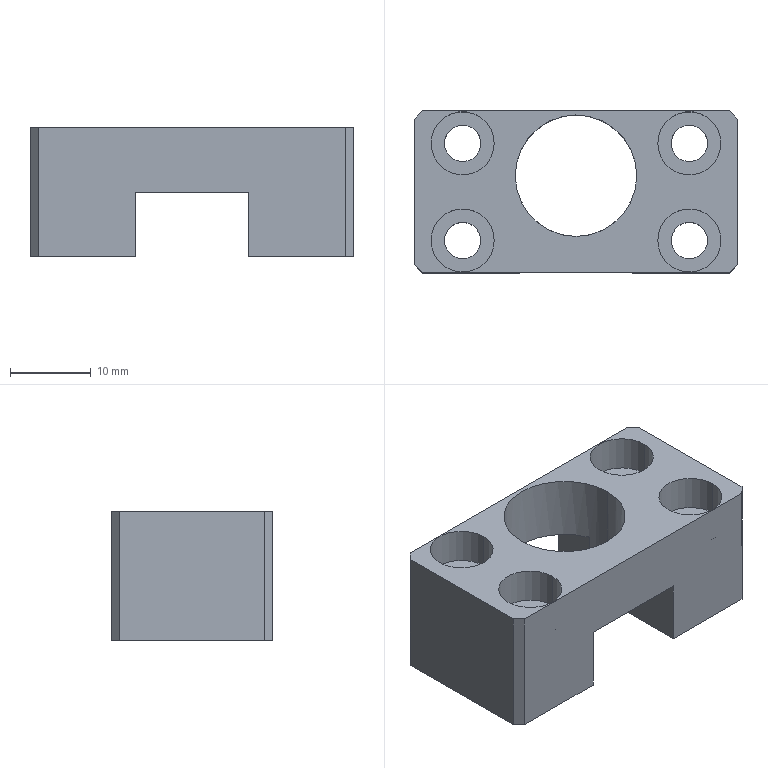Part | SolidWorks | features HoleWzd 2, Chamfer 1, Extrusion 1, ICE 1 | 1 solid | 39 faces | box 40 x 20 x 16 mm | volume 7506 mm3 | plane 21 | cylinder 18 | commonest cylinder face diameters 4.5 x8 7.8 x8 15 x2
STEP:
#1=CARTESIAN_POINT('',(10.1,6.,3.6));
#2=VERTEX_POINT('',#1);
#3=CARTESIAN_POINT('',(17.9,6.,3.6));
#4=VERTEX_POINT('',#3);
#5=CARTESIAN_POINT('',(14.,6.,3.6));
#6=DIRECTION('',(0.,0.,1.));
#7=DIRECTION('',(1.,0.,0.));
#8=AXIS2_PLACEMENT_3D('',#5,#6,#7);
#9=CIRCLE('',#8,3.9);
#10=EDGE_CURVE('',#2,#4,#9,.T.);
#11=ORIENTED_EDGE('',*,*,#10,.F.);
#12=CARTESIAN_POINT('',(10.1,6.,8.));
#13=VERTEX_POINT('',#12);
#14=CARTESIAN_POINT('',(10.1,6.,8.));
#15=DIRECTION('',(0.,0.,1.));
#16=VECTOR('',#15,1000.);
#17=LINE('',#14,#16);
#18=EDGE_CURVE('',#2,#13,#17,.T.);
#19=ORIENTED_EDGE('',*,*,#18,.T.);
#20=CARTESIAN_POINT('',(17.9,6.,8.));
#21=VERTEX_POINT('',#20);
#22=CARTESIAN_POINT('',(14.,6.,8.));
#23=DIRECTION('',(0.,0.,1.));
#24=DIRECTION('',(1.,0.,0.));
#25=AXIS2_PLACEMENT_3D('',#22,#23,#24);
#26=CIRCLE('',#25,3.9);
#27=EDGE_CURVE('',#13,#21,#26,.T.);
#28=ORIENTED_EDGE('',*,*,#27,.T.);
#29=CARTESIAN_POINT('',(17.9,6.,8.));
#30=DIRECTION('',(0.,0.,1.));
#31=VECTOR('',#30,1000.);
#32=LINE('',#29,#31);
#33=EDGE_CURVE('',#4,#21,#32,.T.);
#34=ORIENTED_EDGE('',*,*,#33,.F.);
#35=EDGE_LOOP('',(#11,#19,#28,#34));
#36=FACE_OUTER_BOUND('',#35,.T.);
#37=CARTESIAN_POINT('',(14.,6.,8.));
#38=DIRECTION('',(0.,0.,1.));
#39=DIRECTION('',(1.,0.,0.));
#40=AXIS2_PLACEMENT_3D('',#37,#38,#39);
#41=CYLINDRICAL_SURFACE('',#40,3.9);
#42=ADVANCED_FACE('',(#36),#41,.F.);
#43=CARTESIAN_POINT('',(11.75,6.,-8.));
#44=VERTEX_POINT('',#43);
#45=CARTESIAN_POINT('',(16.25,6.,-8.));
#46=VERTEX_POINT('',#45);
#47=CARTESIAN_POINT('',(14.,6.,-8.));
#48=DIRECTION('',(0.,0.,1.));
#49=DIRECTION('',(1.,0.,0.));
#50=AXIS2_PLACEMENT_3D('',#47,#48,#49);
#51=CIRCLE('',#50,2.25);
#52=EDGE_CURVE('',#44,#46,#51,.T.);
#53=ORIENTED_EDGE('',*,*,#52,.F.);
#54=CARTESIAN_POINT('',(11.75,6.,3.6));
#55=VERTEX_POINT('',#54);
#56=CARTESIAN_POINT('',(11.75,6.,8.));
#57=DIRECTION('',(0.,0.,1.));
#58=VECTOR('',#57,1000.);
#59=LINE('',#56,#58);
#60=EDGE_CURVE('',#44,#55,#59,.T.);
#61=ORIENTED_EDGE('',*,*,#60,.T.);
#62=CARTESIAN_POINT('',(16.25,6.,3.6));
#63=VERTEX_POINT('',#62);
#64=CARTESIAN_POINT('',(14.,6.,3.6));
#65=DIRECTION('',(0.,0.,1.));
#66=DIRECTION('',(1.,0.,0.));
#67=AXIS2_PLACEMENT_3D('',#64,#65,#66);
#68=CIRCLE('',#67,2.25);
#69=EDGE_CURVE('',#55,#63,#68,.T.);
#70=ORIENTED_EDGE('',*,*,#69,.T.);
#71=CARTESIAN_POINT('',(16.25,6.,8.));
#72=DIRECTION('',(0.,0.,1.));
#73=VECTOR('',#72,1000.);
#74=LINE('',#71,#73);
#75=EDGE_CURVE('',#46,#63,#74,.T.);
#76=ORIENTED_EDGE('',*,*,#75,.F.);
#77=EDGE_LOOP('',(#53,#61,#70,#76));
#78=FACE_OUTER_BOUND('',#77,.T.);
#79=CARTESIAN_POINT('',(14.,6.,8.));
#80=DIRECTION('',(0.,0.,1.));
#81=DIRECTION('',(1.,0.,0.));
#82=AXIS2_PLACEMENT_3D('',#79,#80,#81);
#83=CYLINDRICAL_SURFACE('',#82,2.25);
#84=ADVANCED_FACE('',(#78),#83,.F.);
#85=CARTESIAN_POINT('',(-17.9,-6.,3.6));
#86=VERTEX_POINT('',#85);
#87=CARTESIAN_POINT('',(-10.1,-6.,3.6));
#88=VERTEX_POINT('',#87);
#89=CARTESIAN_POINT('',(-14.,-6.,3.6));
#90=DIRECTION('',(0.,0.,1.));
#91=DIRECTION('',(1.,0.,0.));
#92=AXIS2_PLACEMENT_3D('',#89,#90,#91);
#93=CIRCLE('',#92,3.9);
#94=EDGE_CURVE('',#86,#88,#93,.T.);
#95=ORIENTED_EDGE('',*,*,#94,.F.);
#96=CARTESIAN_POINT('',(-17.9,-6.,8.));
#97=VERTEX_POINT('',#96);
#98=CARTESIAN_POINT('',(-17.9,-6.,8.));
#99=DIRECTION('',(0.,0.,1.));
#100=VECTOR('',#99,1000.);
#101=LINE('',#98,#100);
#102=EDGE_CURVE('',#86,#97,#101,.T.);
#103=ORIENTED_EDGE('',*,*,#102,.T.);
#104=CARTESIAN_POINT('',(-10.1,-6.,8.));
#105=VERTEX_POINT('',#104);
#106=CARTESIAN_POINT('',(-14.,-6.,8.));
#107=DIRECTION('',(0.,0.,1.));
#108=DIRECTION('',(1.,0.,0.));
#109=AXIS2_PLACEMENT_3D('',#106,#107,#108);
#110=CIRCLE('',#109,3.9);
#111=EDGE_CURVE('',#97,#105,#110,.T.);
#112=ORIENTED_EDGE('',*,*,#111,.T.);
#113=CARTESIAN_POINT('',(-10.1,-6.,8.));
#114=DIRECTION('',(0.,0.,1.));
#115=VECTOR('',#114,1000.);
#116=LINE('',#113,#115);
#117=EDGE_CURVE('',#88,#105,#116,.T.);
#118=ORIENTED_EDGE('',*,*,#117,.F.);
#119=EDGE_LOOP('',(#95,#103,#112,#118));
#120=FACE_OUTER_BOUND('',#119,.T.);
#121=CARTESIAN_POINT('',(-14.,-6.,8.));
#122=DIRECTION('',(0.,0.,1.));
#123=DIRECTION('',(1.,0.,0.));
#124=AXIS2_PLACEMENT_3D('',#121,#122,#123);
#125=CYLINDRICAL_SURFACE('',#124,3.9);
#126=ADVANCED_FACE('',(#120),#125,.F.);
#127=CARTESIAN_POINT('',(-16.25,-6.,-8.));
#128=VERTEX_POINT('',#127);
#129=CARTESIAN_POINT('',(-11.75,-6.,-8.));
#130=VERTEX_POINT('',#129);
#131=CARTESIAN_POINT('',(-14.,-6.,-8.));
#132=DIRECTION('',(0.,0.,1.));
#133=DIRECTION('',(1.,0.,0.));
#134=AXIS2_PLACEMENT_3D('',#131,#132,#133);
#135=CIRCLE('',#134,2.25);
#136=EDGE_CURVE('',#128,#130,#135,.T.);
#137=ORIENTED_EDGE('',*,*,#136,.F.);
#138=CARTESIAN_POINT('',(-16.25,-6.,3.6));
#139=VERTEX_POINT('',#138);
#140=CARTESIAN_POINT('',(-16.25,-6.,8.));
#141=DIRECTION('',(0.,0.,1.));
#142=VECTOR('',#141,1000.);
#143=LINE('',#140,#142);
#144=EDGE_CURVE('',#128,#139,#143,.T.);
#145=ORIENTED_EDGE('',*,*,#144,.T.);
#146=CARTESIAN_POINT('',(-11.75,-6.,3.6));
#147=VERTEX_POINT('',#146);
#148=CARTESIAN_POINT('',(-14.,-6.,3.6));
#149=DIRECTION('',(0.,0.,1.));
#150=DIRECTION('',(1.,0.,0.));
#151=AXIS2_PLACEMENT_3D('',#148,#149,#150);
#152=CIRCLE('',#151,2.25);
#153=EDGE_CURVE('',#139,#147,#152,.T.);
#154=ORIENTED_EDGE('',*,*,#153,.T.);
#155=CARTESIAN_POINT('',(-11.75,-6.,8.));
#156=DIRECTION('',(0.,0.,1.));
#157=VECTOR('',#156,1000.);
#158=LINE('',#155,#157);
#159=EDGE_CURVE('',#130,#147,#158,.T.);
#160=ORIENTED_EDGE('',*,*,#159,.F.);
#161=EDGE_LOOP('',(#137,#145,#154,#160));
#162=FACE_OUTER_BOUND('',#161,.T.);
#163=CARTESIAN_POINT('',(-14.,-6.,8.));
#164=DIRECTION('',(0.,0.,1.));
#165=DIRECTION('',(1.,0.,0.));
#166=AXIS2_PLACEMENT_3D('',#163,#164,#165);
#167=CYLINDRICAL_SURFACE('',#166,2.25);
#168=ADVANCED_FACE('',(#162),#167,.F.);
#169=CARTESIAN_POINT('',(-17.9,6.,3.6));
#170=VERTEX_POINT('',#169);
#171=CARTESIAN_POINT('',(-10.1,6.,3.6));
#172=VERTEX_POINT('',#171);
#173=CARTESIAN_POINT('',(-14.,6.,3.6));
#174=DIRECTION('',(0.,0.,1.));
#175=DIRECTION('',(1.,0.,0.));
#176=AXIS2_PLACEMENT_3D('',#173,#174,#175);
#177=CIRCLE('',#176,3.9);
#178=EDGE_CURVE('',#170,#172,#177,.T.);
#179=ORIENTED_EDGE('',*,*,#178,.F.);
#180=CARTESIAN_POINT('',(-17.9,6.,8.));
#181=VERTEX_POINT('',#180);
#182=CARTESIAN_POINT('',(-17.9,6.,8.));
#183=DIRECTION('',(0.,0.,1.));
#184=VECTOR('',#183,1000.);
#185=LINE('',#182,#184);
#186=EDGE_CURVE('',#170,#181,#185,.T.);
#187=ORIENTED_EDGE('',*,*,#186,.T.);
#188=CARTESIAN_POINT('',(-10.1,6.,8.));
#189=VERTEX_POINT('',#188);
#190=CARTESIAN_POINT('',(-14.,6.,8.));
#191=DIRECTION('',(0.,0.,1.));
#192=DIRECTION('',(1.,0.,0.));
#193=AXIS2_PLACEMENT_3D('',#190,#191,#192);
#194=CIRCLE('',#193,3.9);
#195=EDGE_CURVE('',#181,#189,#194,.T.);
#196=ORIENTED_EDGE('',*,*,#195,.T.);
#197=CARTESIAN_POINT('',(-10.1,6.,8.));
#198=DIRECTION('',(0.,0.,1.));
#199=VECTOR('',#198,1000.);
#200=LINE('',#197,#199);
#201=EDGE_CURVE('',#172,#189,#200,.T.);
#202=ORIENTED_EDGE('',*,*,#201,.F.);
#203=EDGE_LOOP('',(#179,#187,#196,#202));
#204=FACE_OUTER_BOUND('',#203,.T.);
#205=CARTESIAN_POINT('',(-14.,6.,8.));
#206=DIRECTION('',(0.,0.,1.));
#207=DIRECTION('',(1.,0.,0.));
#208=AXIS2_PLACEMENT_3D('',#205,#206,#207);
#209=CYLINDRICAL_SURFACE('',#208,3.9);
#210=ADVANCED_FACE('',(#204),#209,.F.);
#211=CARTESIAN_POINT('',(-16.25,6.,-8.));
#212=VERTEX_POINT('',#211);
#213=CARTESIAN_POINT('',(-11.75,6.,-8.));
#214=VERTEX_POINT('',#213);
#215=CARTESIAN_POINT('',(-14.,6.,-8.));
#216=DIRECTION('',(0.,0.,1.));
#217=DIRECTION('',(1.,0.,0.));
#218=AXIS2_PLACEMENT_3D('',#215,#216,#217);
#219=CIRCLE('',#218,2.25);
#220=EDGE_CURVE('',#212,#214,#219,.T.);
#221=ORIENTED_EDGE('',*,*,#220,.F.);
#222=CARTESIAN_POINT('',(-16.25,6.,3.6));
#223=VERTEX_POINT('',#222);
#224=CARTESIAN_POINT('',(-16.25,6.,8.));
#225=DIRECTION('',(0.,0.,1.));
#226=VECTOR('',#225,1000.);
#227=LINE('',#224,#226);
#228=EDGE_CURVE('',#212,#223,#227,.T.);
#229=ORIENTED_EDGE('',*,*,#228,.T.);
#230=CARTESIAN_POINT('',(-11.75,6.,3.6));
#231=VERTEX_POINT('',#230);
#232=CARTESIAN_POINT('',(-14.,6.,3.6));
#233=DIRECTION('',(0.,0.,1.));
#234=DIRECTION('',(1.,0.,0.));
#235=AXIS2_PLACEMENT_3D('',#232,#233,#234);
#236=CIRCLE('',#235,2.25);
#237=EDGE_CURVE('',#223,#231,#236,.T.);
#238=ORIENTED_EDGE('',*,*,#237,.T.);
#239=CARTESIAN_POINT('',(-11.75,6.,8.));
#240=DIRECTION('',(0.,0.,1.));
#241=VECTOR('',#240,1000.);
#242=LINE('',#239,#241);
#243=EDGE_CURVE('',#214,#231,#242,.T.);
#244=ORIENTED_EDGE('',*,*,#243,.F.);
#245=EDGE_LOOP('',(#221,#229,#238,#244));
#246=FACE_OUTER_BOUND('',#245,.T.);
#247=CARTESIAN_POINT('',(-14.,6.,8.));
#248=DIRECTION('',(0.,0.,1.));
#249=DIRECTION('',(1.,0.,0.));
#250=AXIS2_PLACEMENT_3D('',#247,#248,#249);
#251=CYLINDRICAL_SURFACE('',#250,2.25);
#252=ADVANCED_FACE('',(#246),#251,.F.);
#253=CARTESIAN_POINT('',(10.1,-6.,3.6));
#254=VERTEX_POINT('',#253);
#255=CARTESIAN_POINT('',(17.9,-6.,3.6));
#256=VERTEX_POINT('',#255);
#257=CARTESIAN_POINT('',(14.,-6.,3.6));
#258=DIRECTION('',(0.,0.,1.));
#259=DIRECTION('',(1.,0.,0.));
#260=AXIS2_PLACEMENT_3D('',#257,#258,#259);
#261=CIRCLE('',#260,3.9);
#262=EDGE_CURVE('',#254,#256,#261,.T.);
#263=ORIENTED_EDGE('',*,*,#262,.F.);
#264=CARTESIAN_POINT('',(10.1,-6.,8.));
#265=VERTEX_POINT('',#264);
#266=CARTESIAN_POINT('',(10.1,-6.,8.));
#267=DIRECTION('',(0.,0.,1.));
#268=VECTOR('',#267,1000.);
#269=LINE('',#266,#268);
#270=EDGE_CURVE('',#254,#265,#269,.T.);
#271=ORIENTED_EDGE('',*,*,#270,.T.);
#272=CARTESIAN_POINT('',(17.9,-6.,8.));
#273=VERTEX_POINT('',#272);
#274=CARTESIAN_POINT('',(14.,-6.,8.));
#275=DIRECTION('',(0.,0.,1.));
#276=DIRECTION('',(1.,0.,0.));
#277=AXIS2_PLACEMENT_3D('',#274,#275,#276);
#278=CIRCLE('',#277,3.9);
#279=EDGE_CURVE('',#265,#273,#278,.T.);
#280=ORIENTED_EDGE('',*,*,#279,.T.);
#281=CARTESIAN_POINT('',(17.9,-6.,8.));
#282=DIRECTION('',(0.,0.,1.));
#283=VECTOR('',#282,1000.);
#284=LINE('',#281,#283);
#285=EDGE_CURVE('',#256,#273,#284,.T.);
#286=ORIENTED_EDGE('',*,*,#285,.F.);
#287=EDGE_LOOP('',(#263,#271,#280,#286));
#288=FACE_OUTER_BOUND('',#287,.T.);
#289=CARTESIAN_POINT('',(14.,-6.,8.));
#290=DIRECTION('',(0.,0.,1.));
#291=DIRECTION('',(1.,0.,0.));
#292=AXIS2_PLACEMENT_3D('',#289,#290,#291);
#293=CYLINDRICAL_SURFACE('',#292,3.9);
#294=ADVANCED_FACE('',(#288),#293,.F.);
#295=CARTESIAN_POINT('',(11.75,-6.,-8.));
#296=VERTEX_POINT('',#295);
#297=CARTESIAN_POINT('',(16.25,-6.,-8.));
#298=VERTEX_POINT('',#297);
#299=CARTESIAN_POINT('',(14.,-6.,-8.));
#300=DIRECTION('',(0.,0.,1.));
#301=DIRECTION('',(1.,0.,0.));
#302=AXIS2_PLACEMENT_3D('',#299,#300,#301);
#303=CIRCLE('',#302,2.25);
#304=EDGE_CURVE('',#296,#298,#303,.T.);
#305=ORIENTED_EDGE('',*,*,#304,.F.);
#306=CARTESIAN_POINT('',(11.75,-6.,3.6));
#307=VERTEX_POINT('',#306);
#308=CARTESIAN_POINT('',(11.75,-6.,8.));
#309=DIRECTION('',(0.,0.,1.));
#310=VECTOR('',#309,1000.);
#311=LINE('',#308,#310);
#312=EDGE_CURVE('',#296,#307,#311,.T.);
#313=ORIENTED_EDGE('',*,*,#312,.T.);
#314=CARTESIAN_POINT('',(16.25,-6.,3.6));
#315=VERTEX_POINT('',#314);
#316=CARTESIAN_POINT('',(14.,-6.,3.6));
#317=DIRECTION('',(0.,0.,1.));
#318=DIRECTION('',(1.,0.,0.));
#319=AXIS2_PLACEMENT_3D('',#316,#317,#318);
#320=CIRCLE('',#319,2.25);
#321=EDGE_CURVE('',#307,#315,#320,.T.);
#322=ORIENTED_EDGE('',*,*,#321,.T.);
#323=CARTESIAN_POINT('',(16.25,-6.,8.));
#324=DIRECTION('',(0.,0.,1.));
#325=VECTOR('',#324,1000.);
#326=LINE('',#323,#325);
#327=EDGE_CURVE('',#298,#315,#326,.T.);
#328=ORIENTED_EDGE('',*,*,#327,.F.);
#329=EDGE_LOOP('',(#305,#313,#322,#328));
#330=FACE_OUTER_BOUND('',#329,.T.);
#331=CARTESIAN_POINT('',(14.,-6.,8.));
#332=DIRECTION('',(0.,0.,1.));
#333=DIRECTION('',(1.,0.,0.));
#334=AXIS2_PLACEMENT_3D('',#331,#332,#333);
#335=CYLINDRICAL_SURFACE('',#334,2.25);
#336=ADVANCED_FACE('',(#330),#335,.F.);
#337=CARTESIAN_POINT('',(-7.,-0.6926,-8.));
#338=VERTEX_POINT('',#337);
#339=CARTESIAN_POINT('',(-7.5,2.,-8.));
#340=VERTEX_POINT('',#339);
#341=CARTESIAN_POINT('',(0.,2.,-8.));
#342=DIRECTION('',(0.,0.,-1.));
#343=DIRECTION('',(-1.,0.,0.));
#344=AXIS2_PLACEMENT_3D('',#341,#342,#343);
#345=CIRCLE('',#344,7.5);
#346=EDGE_CURVE('',#338,#340,#345,.T.);
#347=ORIENTED_EDGE('',*,*,#346,.T.);
#348=CARTESIAN_POINT('',(-7.5,2.,8.));
#349=VERTEX_POINT('',#348);
#350=CARTESIAN_POINT('',(-7.5,2.,8.));
#351=DIRECTION('',(0.,0.,1.));
#352=VECTOR('',#351,1000.);
#353=LINE('',#350,#352);
#354=EDGE_CURVE('',#340,#349,#353,.T.);
#355=ORIENTED_EDGE('',*,*,#354,.T.);
#356=CARTESIAN_POINT('',(7.5,2.,8.));
#357=VERTEX_POINT('',#356);
#358=CARTESIAN_POINT('',(0.,2.,8.));
#359=DIRECTION('',(0.,0.,1.));
#360=DIRECTION('',(1.,0.,0.));
#361=AXIS2_PLACEMENT_3D('',#358,#359,#360);
#362=CIRCLE('',#361,7.5);
#363=EDGE_CURVE('',#349,#357,#362,.T.);
#364=ORIENTED_EDGE('',*,*,#363,.T.);
#365=CARTESIAN_POINT('',(7.5,2.,-8.));
#366=VERTEX_POINT('',#365);
#367=CARTESIAN_POINT('',(7.5,2.,8.));
#368=DIRECTION('',(0.,0.,1.));
#369=VECTOR('',#368,1000.);
#370=LINE('',#367,#369);
#371=EDGE_CURVE('',#366,#357,#370,.T.);
#372=ORIENTED_EDGE('',*,*,#371,.F.);
#373=CARTESIAN_POINT('',(7.,-0.6926,-8.));
#374=VERTEX_POINT('',#373);
#375=CARTESIAN_POINT('',(0.,2.,-8.));
#376=DIRECTION('',(0.,0.,-1.));
#377=DIRECTION('',(-1.,0.,0.));
#378=AXIS2_PLACEMENT_3D('',#375,#376,#377);
#379=CIRCLE('',#378,7.5);
#380=EDGE_CURVE('',#366,#374,#379,.T.);
#381=ORIENTED_EDGE('',*,*,#380,.T.);
#382=CARTESIAN_POINT('',(7.,-0.6926,0.));
#383=VERTEX_POINT('',#382);
#384=CARTESIAN_POINT('',(7.,-0.6926,8.));
#385=DIRECTION('',(0.,0.,1.));
#386=VECTOR('',#385,1000.);
#387=LINE('',#384,#386);
#388=EDGE_CURVE('',#374,#383,#387,.T.);
#389=ORIENTED_EDGE('',*,*,#388,.T.);
#390=CARTESIAN_POINT('',(-7.,-0.6926,0.));
#391=VERTEX_POINT('',#390);
#392=CARTESIAN_POINT('',(0.,2.,0.));
#393=DIRECTION('',(0.,0.,1.));
#394=DIRECTION('',(-1.,0.,0.));
#395=AXIS2_PLACEMENT_3D('',#392,#393,#394);
#396=CIRCLE('',#395,7.5);
#397=EDGE_CURVE('',#391,#383,#396,.T.);
#398=ORIENTED_EDGE('',*,*,#397,.F.);
#399=CARTESIAN_POINT('',(-7.,-0.6926,8.));
#400=DIRECTION('',(0.,0.,-1.));
#401=VECTOR('',#400,1000.);
#402=LINE('',#399,#401);
#403=EDGE_CURVE('',#391,#338,#402,.T.);
#404=ORIENTED_EDGE('',*,*,#403,.T.);
#405=EDGE_LOOP('',(#347,#355,#364,#372,#381,#389,#398,#404));
#406=FACE_OUTER_BOUND('',#405,.T.);
#407=CARTESIAN_POINT('',(0.,2.,8.));
#408=DIRECTION('',(0.,0.,1.));
#409=DIRECTION('',(1.,0.,0.));
#410=AXIS2_PLACEMENT_3D('',#407,#408,#409);
#411=CYLINDRICAL_SURFACE('',#410,7.5);
#412=ADVANCED_FACE('',(#406),#411,.F.);
#413=CARTESIAN_POINT('',(-14.,-6.,-8.));
#414=DIRECTION('',(0.,0.,1.));
#415=DIRECTION('',(1.,0.,0.));
#416=AXIS2_PLACEMENT_3D('',#413,#414,#415);
#417=CIRCLE('',#416,2.25);
#418=EDGE_CURVE('',#130,#128,#417,.T.);
#419=ORIENTED_EDGE('',*,*,#418,.T.);
#420=ORIENTED_EDGE('',*,*,#136,.T.);
#421=EDGE_LOOP('',(#419,#420));
#422=FACE_BOUND('',#421,.T.);
#423=CARTESIAN_POINT('',(-14.,6.,-8.));
#424=DIRECTION('',(0.,0.,1.));
#425=DIRECTION('',(1.,0.,0.));
#426=AXIS2_PLACEMENT_3D('',#423,#424,#425);
#427=CIRCLE('',#426,2.25);
#428=EDGE_CURVE('',#214,#212,#427,.T.);
#429=ORIENTED_EDGE('',*,*,#428,.T.);
#430=ORIENTED_EDGE('',*,*,#220,.T.);
#431=EDGE_LOOP('',(#429,#430));
#432=FACE_BOUND('',#431,.T.);
#433=CARTESIAN_POINT('',(-7.,-10.,-8.));
#434=VERTEX_POINT('',#433);
#435=CARTESIAN_POINT('',(-7.,-15.772,-8.));
#436=DIRECTION('',(0.,1.,0.));
#437=VECTOR('',#436,1000.);
#438=LINE('',#435,#437);
#439=EDGE_CURVE('',#434,#338,#438,.T.);
#440=ORIENTED_EDGE('',*,*,#439,.F.);
#441=CARTESIAN_POINT('',(-19.,-10.,-8.));
#442=VERTEX_POINT('',#441);
#443=CARTESIAN_POINT('',(-20.,-10.,-8.));
#444=DIRECTION('',(1.,0.,0.));
#445=VECTOR('',#444,1000.);
#446=LINE('',#443,#445);
#447=EDGE_CURVE('',#442,#434,#446,.T.);
#448=ORIENTED_EDGE('',*,*,#447,.F.);
#449=CARTESIAN_POINT('',(-20.,-9.,-8.));
#450=VERTEX_POINT('',#449);
#451=CARTESIAN_POINT('',(-14.5,-14.5,-8.));
#452=DIRECTION('',(-0.7071,0.7071,0.));
#453=VECTOR('',#452,1000.);
#454=LINE('',#451,#453);
#455=EDGE_CURVE('',#442,#450,#454,.T.);
#456=ORIENTED_EDGE('',*,*,#455,.T.);
#457=CARTESIAN_POINT('',(-20.,9.,-8.));
#458=VERTEX_POINT('',#457);
#459=CARTESIAN_POINT('',(-20.,-10.,-8.));
#460=DIRECTION('',(0.,-1.,0.));
#461=VECTOR('',#460,1000.);
#462=LINE('',#459,#461);
#463=EDGE_CURVE('',#458,#450,#462,.T.);
#464=ORIENTED_EDGE('',*,*,#463,.F.);
#465=CARTESIAN_POINT('',(-19.,10.,-8.));
#466=VERTEX_POINT('',#465);
#467=CARTESIAN_POINT('',(-14.5,14.5,-8.));
#468=DIRECTION('',(0.7071,0.7071,0.));
#469=VECTOR('',#468,1000.);
#470=LINE('',#467,#469);
#471=EDGE_CURVE('',#458,#466,#470,.T.);
#472=ORIENTED_EDGE('',*,*,#471,.T.);
#473=CARTESIAN_POINT('',(-7.,10.,-8.));
#474=VERTEX_POINT('',#473);
#475=CARTESIAN_POINT('',(-20.,10.,-8.));
#476=DIRECTION('',(-1.,0.,0.));
#477=VECTOR('',#476,1000.);
#478=LINE('',#475,#477);
#479=EDGE_CURVE('',#474,#466,#478,.T.);
#480=ORIENTED_EDGE('',*,*,#479,.F.);
#481=CARTESIAN_POINT('',(-7.,4.693,-8.));
#482=VERTEX_POINT('',#481);
#483=CARTESIAN_POINT('',(-7.,-15.772,-8.));
#484=DIRECTION('',(0.,1.,0.));
#485=VECTOR('',#484,1000.);
#486=LINE('',#483,#485);
#487=EDGE_CURVE('',#482,#474,#486,.T.);
#488=ORIENTED_EDGE('',*,*,#487,.F.);
#489=CARTESIAN_POINT('',(0.,2.,-8.));
#490=DIRECTION('',(0.,0.,-1.));
#491=DIRECTION('',(-1.,0.,0.));
#492=AXIS2_PLACEMENT_3D('',#489,#490,#491);
#493=CIRCLE('',#492,7.5);
#494=EDGE_CURVE('',#340,#482,#493,.T.);
#495=ORIENTED_EDGE('',*,*,#494,.F.);
#496=ORIENTED_EDGE('',*,*,#346,.F.);
#497=EDGE_LOOP('',(#440,#448,#456,#464,#472,#480,#488,#495,#496));
#498=FACE_OUTER_BOUND('',#497,.T.);
#499=CARTESIAN_POINT('',(0.,0.,-8.));
#500=DIRECTION('',(0.,0.,-1.));
#501=DIRECTION('',(-1.,0.,0.));
#502=AXIS2_PLACEMENT_3D('',#499,#500,#501);
#503=PLANE('',#502);
#504=ADVANCED_FACE('',(#422,#432,#498),#503,.T.);
#505=CARTESIAN_POINT('',(20.,-9.,8.));
#506=VERTEX_POINT('',#505);
#507=CARTESIAN_POINT('',(20.,9.,8.));
#508=VERTEX_POINT('',#507);
#509=CARTESIAN_POINT('',(20.,-10.,8.));
#510=DIRECTION('',(0.,1.,0.));
#511=VECTOR('',#510,1000.);
#512=LINE('',#509,#511);
#513=EDGE_CURVE('',#506,#508,#512,.T.);
#514=ORIENTED_EDGE('',*,*,#513,.F.);
#515=CARTESIAN_POINT('',(20.,-9.,-8.));
#516=VERTEX_POINT('',#515);
#517=CARTESIAN_POINT('',(20.,-9.,8.));
#518=DIRECTION('',(0.,0.,-1.));
#519=VECTOR('',#518,1000.);
#520=LINE('',#517,#519);
#521=EDGE_CURVE('',#506,#516,#520,.T.);
#522=ORIENTED_EDGE('',*,*,#521,.T.);
#523=CARTESIAN_POINT('',(20.,9.,-8.));
#524=VERTEX_POINT('',#523);
#525=CARTESIAN_POINT('',(20.,-10.,-8.));
#526=DIRECTION('',(0.,1.,0.));
#527=VECTOR('',#526,1000.);
#528=LINE('',#525,#527);
#529=EDGE_CURVE('',#516,#524,#528,.T.);
#530=ORIENTED_EDGE('',*,*,#529,.T.);
#531=CARTESIAN_POINT('',(20.,9.,8.));
#532=DIRECTION('',(0.,0.,1.));
#533=VECTOR('',#532,1000.);
#534=LINE('',#531,#533);
#535=EDGE_CURVE('',#524,#508,#534,.T.);
#536=ORIENTED_EDGE('',*,*,#535,.T.);
#537=EDGE_LOOP('',(#514,#522,#530,#536));
#538=FACE_OUTER_BOUND('',#537,.T.);
#539=CARTESIAN_POINT('',(20.,-10.,8.));
#540=DIRECTION('',(-1.,0.,0.));
#541=DIRECTION('',(0.,0.,1.));
#542=AXIS2_PLACEMENT_3D('',#539,#540,#541);
#543=PLANE('',#542);
#544=ADVANCED_FACE('',(#538),#543,.F.);
#545=CARTESIAN_POINT('',(-7.,10.,0.));
#546=VERTEX_POINT('',#545);
#547=CARTESIAN_POINT('',(7.,10.,0.));
#548=VERTEX_POINT('',#547);
#549=CARTESIAN_POINT('',(-20.,10.,0.));
#550=DIRECTION('',(1.,0.,0.));
#551=VECTOR('',#550,1000.);
#552=LINE('',#549,#551);
#553=EDGE_CURVE('',#546,#548,#552,.T.);
#554=ORIENTED_EDGE('',*,*,#553,.F.);
#555=CARTESIAN_POINT('',(-7.,10.,8.));
#556=DIRECTION('',(0.,0.,-1.));
#557=VECTOR('',#556,1000.);
#558=LINE('',#555,#557);
#559=EDGE_CURVE('',#546,#474,#558,.T.);
#560=ORIENTED_EDGE('',*,*,#559,.T.);
#561=ORIENTED_EDGE('',*,*,#479,.T.);
#562=CARTESIAN_POINT('',(-19.,10.,8.));
#563=VERTEX_POINT('',#562);
#564=CARTESIAN_POINT('',(-19.,10.,8.));
#565=DIRECTION('',(0.,0.,1.));
#566=VECTOR('',#565,1000.);
#567=LINE('',#564,#566);
#568=EDGE_CURVE('',#466,#563,#567,.T.);
#569=ORIENTED_EDGE('',*,*,#568,.T.);
#570=CARTESIAN_POINT('',(19.,10.,8.));
#571=VERTEX_POINT('',#570);
#572=CARTESIAN_POINT('',(-20.,10.,8.));
#573=DIRECTION('',(-1.,0.,0.));
#574=VECTOR('',#573,1000.);
#575=LINE('',#572,#574);
#576=EDGE_CURVE('',#571,#563,#575,.T.);
#577=ORIENTED_EDGE('',*,*,#576,.F.);
#578=CARTESIAN_POINT('',(19.,10.,-8.));
#579=VERTEX_POINT('',#578);
#580=CARTESIAN_POINT('',(19.,10.,8.));
#581=DIRECTION('',(0.,0.,-1.));
#582=VECTOR('',#581,1000.);
#583=LINE('',#580,#582);
#584=EDGE_CURVE('',#571,#579,#583,.T.);
#585=ORIENTED_EDGE('',*,*,#584,.T.);
#586=CARTESIAN_POINT('',(7.,10.,-8.));
#587=VERTEX_POINT('',#586);
#588=CARTESIAN_POINT('',(-20.,10.,-8.));
#589=DIRECTION('',(-1.,0.,0.));
#590=VECTOR('',#589,1000.);
#591=LINE('',#588,#590);
#592=EDGE_CURVE('',#579,#587,#591,.T.);
#593=ORIENTED_EDGE('',*,*,#592,.T.);
#594=CARTESIAN_POINT('',(7.,10.,8.));
#595=DIRECTION('',(0.,0.,1.));
#596=VECTOR('',#595,1000.);
#597=LINE('',#594,#596);
#598=EDGE_CURVE('',#587,#548,#597,.T.);
#599=ORIENTED_EDGE('',*,*,#598,.T.);
#600=EDGE_LOOP('',(#554,#560,#561,#569,#577,#585,#593,#599));
#601=FACE_OUTER_BOUND('',#600,.T.);
#602=CARTESIAN_POINT('',(-20.,10.,8.));
#603=DIRECTION('',(0.,-1.,0.));
#604=DIRECTION('',(0.,0.,-1.));
#605=AXIS2_PLACEMENT_3D('',#602,#603,#604);
#606=PLANE('',#605);
#607=ADVANCED_FACE('',(#601),#606,.F.);
#608=ORIENTED_EDGE('',*,*,#463,.T.);
#609=CARTESIAN_POINT('',(-20.,-9.,8.));
#610=VERTEX_POINT('',#609);
#611=CARTESIAN_POINT('',(-20.,-9.,8.));
#612=DIRECTION('',(0.,0.,1.));
#613=VECTOR('',#612,1000.);
#614=LINE('',#611,#613);
#615=EDGE_CURVE('',#450,#610,#614,.T.);
#616=ORIENTED_EDGE('',*,*,#615,.T.);
#617=CARTESIAN_POINT('',(-20.,9.,8.));
#618=VERTEX_POINT('',#617);
#619=CARTESIAN_POINT('',(-20.,-10.,8.));
#620=DIRECTION('',(0.,-1.,0.));
#621=VECTOR('',#620,1000.);
#622=LINE('',#619,#621);
#623=EDGE_CURVE('',#618,#610,#622,.T.);
#624=ORIENTED_EDGE('',*,*,#623,.F.);
#625=CARTESIAN_POINT('',(-20.,9.,8.));
#626=DIRECTION('',(0.,0.,-1.));
#627=VECTOR('',#626,1000.);
#628=LINE('',#625,#627);
#629=EDGE_CURVE('',#618,#458,#628,.T.);
#630=ORIENTED_EDGE('',*,*,#629,.T.);
#631=EDGE_LOOP('',(#608,#616,#624,#630));
#632=FACE_OUTER_BOUND('',#631,.T.);
#633=CARTESIAN_POINT('',(-20.,-10.,8.));
#634=DIRECTION('',(1.,0.,0.));
#635=DIRECTION('',(0.,0.,-1.));
#636=AXIS2_PLACEMENT_3D('',#633,#634,#635);
#637=PLANE('',#636);
#638=ADVANCED_FACE('',(#632),#637,.F.);
#639=ORIENTED_EDGE('',*,*,#447,.T.);
#640=CARTESIAN_POINT('',(-7.,-10.,0.));
#641=VERTEX_POINT('',#640);
#642=CARTESIAN_POINT('',(-7.,-10.,8.));
#643=DIRECTION('',(0.,0.,1.));
#644=VECTOR('',#643,1000.);
#645=LINE('',#642,#644);
#646=EDGE_CURVE('',#434,#641,#645,.T.);
#647=ORIENTED_EDGE('',*,*,#646,.T.);
#648=CARTESIAN_POINT('',(7.,-10.,0.));
#649=VERTEX_POINT('',#648);
#650=CARTESIAN_POINT('',(-20.,-10.,0.));
#651=DIRECTION('',(-1.,0.,0.));
#652=VECTOR('',#651,1000.);
#653=LINE('',#650,#652);
#654=EDGE_CURVE('',#649,#641,#653,.T.);
#655=ORIENTED_EDGE('',*,*,#654,.F.);
#656=CARTESIAN_POINT('',(7.,-10.,-8.));
#657=VERTEX_POINT('',#656);
#658=CARTESIAN_POINT('',(7.,-10.,8.));
#659=DIRECTION('',(0.,0.,-1.));
#660=VECTOR('',#659,1000.);
#661=LINE('',#658,#660);
#662=EDGE_CURVE('',#649,#657,#661,.T.);
#663=ORIENTED_EDGE('',*,*,#662,.T.);
#664=CARTESIAN_POINT('',(19.,-10.,-8.));
#665=VERTEX_POINT('',#664);
#666=CARTESIAN_POINT('',(-20.,-10.,-8.));
#667=DIRECTION('',(1.,0.,0.));
#668=VECTOR('',#667,1000.);
#669=LINE('',#666,#668);
#670=EDGE_CURVE('',#657,#665,#669,.T.);
#671=ORIENTED_EDGE('',*,*,#670,.T.);
#672=CARTESIAN_POINT('',(19.,-10.,8.));
#673=VERTEX_POINT('',#672);
#674=CARTESIAN_POINT('',(19.,-10.,8.));
#675=DIRECTION('',(0.,0.,1.));
#676=VECTOR('',#675,1000.);
#677=LINE('',#674,#676);
#678=EDGE_CURVE('',#665,#673,#677,.T.);
#679=ORIENTED_EDGE('',*,*,#678,.T.);
#680=CARTESIAN_POINT('',(-19.,-10.,8.));
#681=VERTEX_POINT('',#680);
#682=CARTESIAN_POINT('',(-20.,-10.,8.));
#683=DIRECTION('',(1.,0.,0.));
#684=VECTOR('',#683,1000.);
#685=LINE('',#682,#684);
#686=EDGE_CURVE('',#681,#673,#685,.T.);
#687=ORIENTED_EDGE('',*,*,#686,.F.);
#688=CARTESIAN_POINT('',(-19.,-10.,8.));
#689=DIRECTION('',(0.,0.,-1.));
#690=VECTOR('',#689,1000.);
#691=LINE('',#688,#690);
#692=EDGE_CURVE('',#681,#442,#691,.T.);
#693=ORIENTED_EDGE('',*,*,#692,.T.);
#694=EDGE_LOOP('',(#639,#647,#655,#663,#671,#679,#687,#693));
#695=FACE_OUTER_BOUND('',#694,.T.);
#696=CARTESIAN_POINT('',(-20.,-10.,8.));
#697=DIRECTION('',(0.,1.,0.));
#698=DIRECTION('',(0.,0.,1.));
#699=AXIS2_PLACEMENT_3D('',#696,#697,#698);
#700=PLANE('',#699);
#701=ADVANCED_FACE('',(#695),#700,.F.);
#702=CARTESIAN_POINT('',(14.,6.,8.));
#703=DIRECTION('',(0.,0.,1.));
#704=DIRECTION('',(1.,0.,0.));
#705=AXIS2_PLACEMENT_3D('',#702,#703,#704);
#706=CIRCLE('',#705,3.9);
#707=EDGE_CURVE('',#21,#13,#706,.T.);
#708=ORIENTED_EDGE('',*,*,#707,.F.);
#709=ORIENTED_EDGE('',*,*,#27,.F.);
#710=EDGE_LOOP('',(#708,#709));
#711=FACE_BOUND('',#710,.T.);
#712=CARTESIAN_POINT('',(-14.,-6.,8.));
#713=DIRECTION('',(0.,0.,1.));
#714=DIRECTION('',(1.,0.,0.));
#715=AXIS2_PLACEMENT_3D('',#712,#713,#714);
#716=CIRCLE('',#715,3.9);
#717=EDGE_CURVE('',#105,#97,#716,.T.);
#718=ORIENTED_EDGE('',*,*,#717,.F.);
#719=ORIENTED_EDGE('',*,*,#111,.F.);
#720=EDGE_LOOP('',(#718,#719));
#721=FACE_BOUND('',#720,.T.);
#722=CARTESIAN_POINT('',(-14.,6.,8.));
#723=DIRECTION('',(0.,0.,1.));
#724=DIRECTION('',(1.,0.,0.));
#725=AXIS2_PLACEMENT_3D('',#722,#723,#724);
#726=CIRCLE('',#725,3.9);
#727=EDGE_CURVE('',#189,#181,#726,.T.);
#728=ORIENTED_EDGE('',*,*,#727,.F.);
#729=ORIENTED_EDGE('',*,*,#195,.F.);
#730=EDGE_LOOP('',(#728,#729));
#731=FACE_BOUND('',#730,.T.);
#732=CARTESIAN_POINT('',(14.,-6.,8.));
#733=DIRECTION('',(0.,0.,1.));
#734=DIRECTION('',(1.,0.,0.));
#735=AXIS2_PLACEMENT_3D('',#732,#733,#734);
#736=CIRCLE('',#735,3.9);
#737=EDGE_CURVE('',#273,#265,#736,.T.);
#738=ORIENTED_EDGE('',*,*,#737,.F.);
#739=ORIENTED_EDGE('',*,*,#279,.F.);
#740=EDGE_LOOP('',(#738,#739));
#741=FACE_BOUND('',#740,.T.);
#742=CARTESIAN_POINT('',(0.,2.,8.));
#743=DIRECTION('',(0.,0.,1.));
#744=DIRECTION('',(1.,0.,0.));
#745=AXIS2_PLACEMENT_3D('',#742,#743,#744);
#746=CIRCLE('',#745,7.5);
#747=EDGE_CURVE('',#357,#349,#746,.T.);
#748=ORIENTED_EDGE('',*,*,#747,.F.);
#749=ORIENTED_EDGE('',*,*,#363,.F.);
#750=EDGE_LOOP('',(#748,#749));
#751=FACE_BOUND('',#750,.T.);
#752=ORIENTED_EDGE('',*,*,#623,.T.);
#753=CARTESIAN_POINT('',(-19.,-10.,8.));
#754=DIRECTION('',(0.7071,-0.7071,0.));
#755=VECTOR('',#754,1000.);
#756=LINE('',#753,#755);
#757=EDGE_CURVE('',#610,#681,#756,.T.);
#758=ORIENTED_EDGE('',*,*,#757,.T.);
#759=ORIENTED_EDGE('',*,*,#686,.T.);
#760=CARTESIAN_POINT('',(20.,-9.,8.));
#761=DIRECTION('',(0.7071,0.7071,0.));
#762=VECTOR('',#761,1000.);
#763=LINE('',#760,#762);
#764=EDGE_CURVE('',#673,#506,#763,.T.);
#765=ORIENTED_EDGE('',*,*,#764,.T.);
#766=ORIENTED_EDGE('',*,*,#513,.T.);
#767=CARTESIAN_POINT('',(19.,10.,8.));
#768=DIRECTION('',(-0.7071,0.7071,0.));
#769=VECTOR('',#768,1000.);
#770=LINE('',#767,#769);
#771=EDGE_CURVE('',#508,#571,#770,.T.);
#772=ORIENTED_EDGE('',*,*,#771,.T.);
#773=ORIENTED_EDGE('',*,*,#576,.T.);
#774=CARTESIAN_POINT('',(-20.,9.,8.));
#775=DIRECTION('',(-0.7071,-0.7071,0.));
#776=VECTOR('',#775,1000.);
#777=LINE('',#774,#776);
#778=EDGE_CURVE('',#563,#618,#777,.T.);
#779=ORIENTED_EDGE('',*,*,#778,.T.);
#780=EDGE_LOOP('',(#752,#758,#759,#765,#766,#772,#773,#779));
#781=FACE_OUTER_BOUND('',#780,.T.);
#782=CARTESIAN_POINT('',(0.,0.,8.));
#783=DIRECTION('',(0.,0.,-1.));
#784=DIRECTION('',(-1.,0.,0.));
#785=AXIS2_PLACEMENT_3D('',#782,#783,#784);
#786=PLANE('',#785);
#787=ADVANCED_FACE('',(#711,#721,#731,#741,#751,#781),#786,.F.);
#788=CARTESIAN_POINT('',(14.,6.,-8.));
#789=DIRECTION('',(0.,0.,1.));
#790=DIRECTION('',(1.,0.,0.));
#791=AXIS2_PLACEMENT_3D('',#788,#789,#790);
#792=CIRCLE('',#791,2.25);
#793=EDGE_CURVE('',#46,#44,#792,.T.);
#794=ORIENTED_EDGE('',*,*,#793,.T.);
#795=ORIENTED_EDGE('',*,*,#52,.T.);
#796=EDGE_LOOP('',(#794,#795));
#797=FACE_BOUND('',#796,.T.);
#798=CARTESIAN_POINT('',(14.,-6.,-8.));
#799=DIRECTION('',(0.,0.,1.));
#800=DIRECTION('',(1.,0.,0.));
#801=AXIS2_PLACEMENT_3D('',#798,#799,#800);
#802=CIRCLE('',#801,2.25);
#803=EDGE_CURVE('',#298,#296,#802,.T.);
#804=ORIENTED_EDGE('',*,*,#803,.T.);
#805=ORIENTED_EDGE('',*,*,#304,.T.);
#806=EDGE_LOOP('',(#804,#805));
#807=FACE_BOUND('',#806,.T.);
#808=CARTESIAN_POINT('',(7.,4.693,-8.));
#809=VERTEX_POINT('',#808);
#810=CARTESIAN_POINT('',(7.,-14.986,-8.));
#811=DIRECTION('',(0.,-1.,0.));
#812=VECTOR('',#811,1000.);
#813=LINE('',#810,#812);
#814=EDGE_CURVE('',#587,#809,#813,.T.);
#815=ORIENTED_EDGE('',*,*,#814,.F.);
#816=ORIENTED_EDGE('',*,*,#592,.F.);
#817=CARTESIAN_POINT('',(14.5,14.5,-8.));
#818=DIRECTION('',(0.7071,-0.7071,0.));
#819=VECTOR('',#818,1000.);
#820=LINE('',#817,#819);
#821=EDGE_CURVE('',#579,#524,#820,.T.);
#822=ORIENTED_EDGE('',*,*,#821,.T.);
#823=ORIENTED_EDGE('',*,*,#529,.F.);
#824=CARTESIAN_POINT('',(14.5,-14.5,-8.));
#825=DIRECTION('',(-0.7071,-0.7071,0.));
#826=VECTOR('',#825,1000.);
#827=LINE('',#824,#826);
#828=EDGE_CURVE('',#516,#665,#827,.T.);
#829=ORIENTED_EDGE('',*,*,#828,.T.);
#830=ORIENTED_EDGE('',*,*,#670,.F.);
#831=CARTESIAN_POINT('',(7.,-14.986,-8.));
#832=DIRECTION('',(0.,-1.,0.));
#833=VECTOR('',#832,1000.);
#834=LINE('',#831,#833);
#835=EDGE_CURVE('',#374,#657,#834,.T.);
#836=ORIENTED_EDGE('',*,*,#835,.F.);
#837=ORIENTED_EDGE('',*,*,#380,.F.);
#838=CARTESIAN_POINT('',(0.,2.,-8.));
#839=DIRECTION('',(0.,0.,-1.));
#840=DIRECTION('',(-1.,0.,0.));
#841=AXIS2_PLACEMENT_3D('',#838,#839,#840);
#842=CIRCLE('',#841,7.5);
#843=EDGE_CURVE('',#809,#366,#842,.T.);
#844=ORIENTED_EDGE('',*,*,#843,.F.);
#845=EDGE_LOOP('',(#815,#816,#822,#823,#829,#830,#836,#837,#844));
#846=FACE_OUTER_BOUND('',#845,.T.);
#847=CARTESIAN_POINT('',(0.,0.,-8.));
#848=DIRECTION('',(0.,0.,-1.));
#849=DIRECTION('',(-1.,0.,0.));
#850=AXIS2_PLACEMENT_3D('',#847,#848,#849);
#851=PLANE('',#850);
#852=ADVANCED_FACE('',(#797,#807,#846),#851,.T.);
#853=ORIENTED_EDGE('',*,*,#757,.F.);
#854=ORIENTED_EDGE('',*,*,#615,.F.);
#855=ORIENTED_EDGE('',*,*,#455,.F.);
#856=ORIENTED_EDGE('',*,*,#692,.F.);
#857=EDGE_LOOP('',(#853,#854,#855,#856));
#858=FACE_OUTER_BOUND('',#857,.T.);
#859=CARTESIAN_POINT('',(-19.,-10.,8.));
#860=DIRECTION('',(0.7071,0.7071,0.));
#861=DIRECTION('',(0.,0.,-1.));
#862=AXIS2_PLACEMENT_3D('',#859,#860,#861);
#863=PLANE('',#862);
#864=ADVANCED_FACE('',(#858),#863,.F.);
#865=ORIENTED_EDGE('',*,*,#764,.F.);
#866=ORIENTED_EDGE('',*,*,#678,.F.);
#867=ORIENTED_EDGE('',*,*,#828,.F.);
#868=ORIENTED_EDGE('',*,*,#521,.F.);
#869=EDGE_LOOP('',(#865,#866,#867,#868));
#870=FACE_OUTER_BOUND('',#869,.T.);
#871=CARTESIAN_POINT('',(20.,-9.,8.));
#872=DIRECTION('',(-0.7071,0.7071,0.));
#873=DIRECTION('',(0.,0.,-1.));
#874=AXIS2_PLACEMENT_3D('',#871,#872,#873);
#875=PLANE('',#874);
#876=ADVANCED_FACE('',(#870),#875,.F.);
#877=ORIENTED_EDGE('',*,*,#771,.F.);
#878=ORIENTED_EDGE('',*,*,#535,.F.);
#879=ORIENTED_EDGE('',*,*,#821,.F.);
#880=ORIENTED_EDGE('',*,*,#584,.F.);
#881=EDGE_LOOP('',(#877,#878,#879,#880));
#882=FACE_OUTER_BOUND('',#881,.T.);
#883=CARTESIAN_POINT('',(19.,10.,8.));
#884=DIRECTION('',(-0.7071,-0.7071,0.));
#885=DIRECTION('',(0.,0.,-1.));
#886=AXIS2_PLACEMENT_3D('',#883,#884,#885);
#887=PLANE('',#886);
#888=ADVANCED_FACE('',(#882),#887,.F.);
#889=ORIENTED_EDGE('',*,*,#778,.F.);
#890=ORIENTED_EDGE('',*,*,#568,.F.);
#891=ORIENTED_EDGE('',*,*,#471,.F.);
#892=ORIENTED_EDGE('',*,*,#629,.F.);
#893=EDGE_LOOP('',(#889,#890,#891,#892));
#894=FACE_OUTER_BOUND('',#893,.T.);
#895=CARTESIAN_POINT('',(-20.,9.,8.));
#896=DIRECTION('',(0.7071,-0.7071,0.));
#897=DIRECTION('',(0.,0.,-1.));
#898=AXIS2_PLACEMENT_3D('',#895,#896,#897);
#899=PLANE('',#898);
#900=ADVANCED_FACE('',(#894),#899,.F.);
#901=ORIENTED_EDGE('',*,*,#354,.F.);
#902=ORIENTED_EDGE('',*,*,#494,.T.);
#903=CARTESIAN_POINT('',(-7.,4.693,0.));
#904=VERTEX_POINT('',#903);
#905=CARTESIAN_POINT('',(-7.,4.693,8.));
#906=DIRECTION('',(0.,0.,1.));
#907=VECTOR('',#906,1000.);
#908=LINE('',#905,#907);
#909=EDGE_CURVE('',#482,#904,#908,.T.);
#910=ORIENTED_EDGE('',*,*,#909,.T.);
#911=CARTESIAN_POINT('',(7.,4.693,0.));
#912=VERTEX_POINT('',#911);
#913=CARTESIAN_POINT('',(0.,2.,0.));
#914=DIRECTION('',(0.,0.,1.));
#915=DIRECTION('',(-1.,0.,0.));
#916=AXIS2_PLACEMENT_3D('',#913,#914,#915);
#917=CIRCLE('',#916,7.5);
#918=EDGE_CURVE('',#912,#904,#917,.T.);
#919=ORIENTED_EDGE('',*,*,#918,.F.);
#920=CARTESIAN_POINT('',(7.,4.693,8.));
#921=DIRECTION('',(0.,0.,-1.));
#922=VECTOR('',#921,1000.);
#923=LINE('',#920,#922);
#924=EDGE_CURVE('',#912,#809,#923,.T.);
#925=ORIENTED_EDGE('',*,*,#924,.T.);
#926=ORIENTED_EDGE('',*,*,#843,.T.);
#927=ORIENTED_EDGE('',*,*,#371,.T.);
#928=ORIENTED_EDGE('',*,*,#747,.T.);
#929=EDGE_LOOP('',(#901,#902,#910,#919,#925,#926,#927,#928));
#930=FACE_OUTER_BOUND('',#929,.T.);
#931=CARTESIAN_POINT('',(0.,2.,8.));
#932=DIRECTION('',(0.,0.,1.));
#933=DIRECTION('',(1.,0.,0.));
#934=AXIS2_PLACEMENT_3D('',#931,#932,#933);
#935=CYLINDRICAL_SURFACE('',#934,7.5);
#936=ADVANCED_FACE('',(#930),#935,.F.);
#937=ORIENTED_EDGE('',*,*,#553,.T.);
#938=CARTESIAN_POINT('',(7.,-14.986,0.));
#939=DIRECTION('',(0.,-1.,0.));
#940=VECTOR('',#939,1000.);
#941=LINE('',#938,#940);
#942=EDGE_CURVE('',#548,#912,#941,.T.);
#943=ORIENTED_EDGE('',*,*,#942,.T.);
#944=ORIENTED_EDGE('',*,*,#918,.T.);
#945=CARTESIAN_POINT('',(-7.,-15.772,0.));
#946=DIRECTION('',(0.,1.,0.));
#947=VECTOR('',#946,1000.);
#948=LINE('',#945,#947);
#949=EDGE_CURVE('',#904,#546,#948,.T.);
#950=ORIENTED_EDGE('',*,*,#949,.T.);
#951=EDGE_LOOP('',(#937,#943,#944,#950));
#952=FACE_OUTER_BOUND('',#951,.T.);
#953=CARTESIAN_POINT('',(0.,0.,0.));
#954=DIRECTION('',(0.,0.,-1.));
#955=DIRECTION('',(-1.,0.,0.));
#956=AXIS2_PLACEMENT_3D('',#953,#954,#955);
#957=PLANE('',#956);
#958=ADVANCED_FACE('',(#952),#957,.T.);
#959=ORIENTED_EDGE('',*,*,#814,.T.);
#960=ORIENTED_EDGE('',*,*,#924,.F.);
#961=ORIENTED_EDGE('',*,*,#942,.F.);
#962=ORIENTED_EDGE('',*,*,#598,.F.);
#963=EDGE_LOOP('',(#959,#960,#961,#962));
#964=FACE_OUTER_BOUND('',#963,.T.);
#965=CARTESIAN_POINT('',(7.,-14.986,0.));
#966=DIRECTION('',(1.,0.,0.));
#967=DIRECTION('',(0.,0.,-1.));
#968=AXIS2_PLACEMENT_3D('',#965,#966,#967);
#969=PLANE('',#968);
#970=ADVANCED_FACE('',(#964),#969,.F.);
#971=ORIENTED_EDGE('',*,*,#949,.F.);
#972=ORIENTED_EDGE('',*,*,#909,.F.);
#973=ORIENTED_EDGE('',*,*,#487,.T.);
#974=ORIENTED_EDGE('',*,*,#559,.F.);
#975=EDGE_LOOP('',(#971,#972,#973,#974));
#976=FACE_OUTER_BOUND('',#975,.T.);
#977=CARTESIAN_POINT('',(-7.,-15.772,0.));
#978=DIRECTION('',(-1.,0.,0.));
#979=DIRECTION('',(0.,0.,1.));
#980=AXIS2_PLACEMENT_3D('',#977,#978,#979);
#981=PLANE('',#980);
#982=ADVANCED_FACE('',(#976),#981,.F.);
#983=ORIENTED_EDGE('',*,*,#439,.T.);
#984=ORIENTED_EDGE('',*,*,#403,.F.);
#985=CARTESIAN_POINT('',(-7.,-15.772,0.));
#986=DIRECTION('',(0.,1.,0.));
#987=VECTOR('',#986,1000.);
#988=LINE('',#985,#987);
#989=EDGE_CURVE('',#641,#391,#988,.T.);
#990=ORIENTED_EDGE('',*,*,#989,.F.);
#991=ORIENTED_EDGE('',*,*,#646,.F.);
#992=EDGE_LOOP('',(#983,#984,#990,#991));
#993=FACE_OUTER_BOUND('',#992,.T.);
#994=CARTESIAN_POINT('',(-7.,-15.772,0.));
#995=DIRECTION('',(-1.,0.,0.));
#996=DIRECTION('',(0.,0.,1.));
#997=AXIS2_PLACEMENT_3D('',#994,#995,#996);
#998=PLANE('',#997);
#999=ADVANCED_FACE('',(#993),#998,.F.);
#1000=CARTESIAN_POINT('',(7.,-14.986,0.));
#1001=DIRECTION('',(0.,-1.,0.));
#1002=VECTOR('',#1001,1000.);
#1003=LINE('',#1000,#1002);
#1004=EDGE_CURVE('',#383,#649,#1003,.T.);
#1005=ORIENTED_EDGE('',*,*,#1004,.F.);
#1006=ORIENTED_EDGE('',*,*,#388,.F.);
#1007=ORIENTED_EDGE('',*,*,#835,.T.);
#1008=ORIENTED_EDGE('',*,*,#662,.F.);
#1009=EDGE_LOOP('',(#1005,#1006,#1007,#1008));
#1010=FACE_OUTER_BOUND('',#1009,.T.);
#1011=CARTESIAN_POINT('',(7.,-14.986,0.));
#1012=DIRECTION('',(1.,0.,0.));
#1013=DIRECTION('',(0.,0.,-1.));
#1014=AXIS2_PLACEMENT_3D('',#1011,#1012,#1013);
#1015=PLANE('',#1014);
#1016=ADVANCED_FACE('',(#1010),#1015,.F.);
#1017=ORIENTED_EDGE('',*,*,#654,.T.);
#1018=ORIENTED_EDGE('',*,*,#989,.T.);
#1019=ORIENTED_EDGE('',*,*,#397,.T.);
#1020=ORIENTED_EDGE('',*,*,#1004,.T.);
#1021=EDGE_LOOP('',(#1017,#1018,#1019,#1020));
#1022=FACE_OUTER_BOUND('',#1021,.T.);
#1023=CARTESIAN_POINT('',(0.,0.,0.));
#1024=DIRECTION('',(0.,0.,-1.));
#1025=DIRECTION('',(-1.,0.,0.));
#1026=AXIS2_PLACEMENT_3D('',#1023,#1024,#1025);
#1027=PLANE('',#1026);
#1028=ADVANCED_FACE('',(#1022),#1027,.T.);
#1029=ORIENTED_EDGE('',*,*,#312,.F.);
#1030=ORIENTED_EDGE('',*,*,#803,.F.);
#1031=ORIENTED_EDGE('',*,*,#327,.T.);
#1032=CARTESIAN_POINT('',(14.,-6.,3.6));
#1033=DIRECTION('',(0.,0.,1.));
#1034=DIRECTION('',(1.,0.,0.));
#1035=AXIS2_PLACEMENT_3D('',#1032,#1033,#1034);
#1036=CIRCLE('',#1035,2.25);
#1037=EDGE_CURVE('',#315,#307,#1036,.T.);
#1038=ORIENTED_EDGE('',*,*,#1037,.T.);
#1039=EDGE_LOOP('',(#1029,#1030,#1031,#1038));
#1040=FACE_OUTER_BOUND('',#1039,.T.);
#1041=CARTESIAN_POINT('',(14.,-6.,8.));
#1042=DIRECTION('',(0.,0.,1.));
#1043=DIRECTION('',(1.,0.,0.));
#1044=AXIS2_PLACEMENT_3D('',#1041,#1042,#1043);
#1045=CYLINDRICAL_SURFACE('',#1044,2.25);
#1046=ADVANCED_FACE('',(#1040),#1045,.F.);
#1047=ORIENTED_EDGE('',*,*,#1037,.F.);
#1048=ORIENTED_EDGE('',*,*,#321,.F.);
#1049=EDGE_LOOP('',(#1047,#1048));
#1050=FACE_BOUND('',#1049,.T.);
#1051=CARTESIAN_POINT('',(14.,-6.,3.6));
#1052=DIRECTION('',(0.,0.,1.));
#1053=DIRECTION('',(1.,0.,0.));
#1054=AXIS2_PLACEMENT_3D('',#1051,#1052,#1053);
#1055=CIRCLE('',#1054,3.9);
#1056=EDGE_CURVE('',#256,#254,#1055,.T.);
#1057=ORIENTED_EDGE('',*,*,#1056,.T.);
#1058=ORIENTED_EDGE('',*,*,#262,.T.);
#1059=EDGE_LOOP('',(#1057,#1058));
#1060=FACE_OUTER_BOUND('',#1059,.T.);
#1061=CARTESIAN_POINT('',(16.25,-6.,3.6));
#1062=DIRECTION('',(0.,0.,-1.));
#1063=DIRECTION('',(-1.,0.,0.));
#1064=AXIS2_PLACEMENT_3D('',#1061,#1062,#1063);
#1065=PLANE('',#1064);
#1066=ADVANCED_FACE('',(#1050,#1060),#1065,.F.);
#1067=ORIENTED_EDGE('',*,*,#270,.F.);
#1068=ORIENTED_EDGE('',*,*,#1056,.F.);
#1069=ORIENTED_EDGE('',*,*,#285,.T.);
#1070=ORIENTED_EDGE('',*,*,#737,.T.);
#1071=EDGE_LOOP('',(#1067,#1068,#1069,#1070));
#1072=FACE_OUTER_BOUND('',#1071,.T.);
#1073=CARTESIAN_POINT('',(14.,-6.,8.));
#1074=DIRECTION('',(0.,0.,1.));
#1075=DIRECTION('',(1.,0.,0.));
#1076=AXIS2_PLACEMENT_3D('',#1073,#1074,#1075);
#1077=CYLINDRICAL_SURFACE('',#1076,3.9);
#1078=ADVANCED_FACE('',(#1072),#1077,.F.);
#1079=ORIENTED_EDGE('',*,*,#228,.F.);
#1080=ORIENTED_EDGE('',*,*,#428,.F.);
#1081=ORIENTED_EDGE('',*,*,#243,.T.);
#1082=CARTESIAN_POINT('',(-14.,6.,3.6));
#1083=DIRECTION('',(0.,0.,1.));
#1084=DIRECTION('',(1.,0.,0.));
#1085=AXIS2_PLACEMENT_3D('',#1082,#1083,#1084);
#1086=CIRCLE('',#1085,2.25);
#1087=EDGE_CURVE('',#231,#223,#1086,.T.);
#1088=ORIENTED_EDGE('',*,*,#1087,.T.);
#1089=EDGE_LOOP('',(#1079,#1080,#1081,#1088));
#1090=FACE_OUTER_BOUND('',#1089,.T.);
#1091=CARTESIAN_POINT('',(-14.,6.,8.));
#1092=DIRECTION('',(0.,0.,1.));
#1093=DIRECTION('',(1.,0.,0.));
#1094=AXIS2_PLACEMENT_3D('',#1091,#1092,#1093);
#1095=CYLINDRICAL_SURFACE('',#1094,2.25);
#1096=ADVANCED_FACE('',(#1090),#1095,.F.);
#1097=ORIENTED_EDGE('',*,*,#1087,.F.);
#1098=ORIENTED_EDGE('',*,*,#237,.F.);
#1099=EDGE_LOOP('',(#1097,#1098));
#1100=FACE_BOUND('',#1099,.T.);
#1101=CARTESIAN_POINT('',(-14.,6.,3.6));
#1102=DIRECTION('',(0.,0.,1.));
#1103=DIRECTION('',(1.,0.,0.));
#1104=AXIS2_PLACEMENT_3D('',#1101,#1102,#1103);
#1105=CIRCLE('',#1104,3.9);
#1106=EDGE_CURVE('',#172,#170,#1105,.T.);
#1107=ORIENTED_EDGE('',*,*,#1106,.T.);
#1108=ORIENTED_EDGE('',*,*,#178,.T.);
#1109=EDGE_LOOP('',(#1107,#1108));
#1110=FACE_OUTER_BOUND('',#1109,.T.);
#1111=CARTESIAN_POINT('',(-11.75,6.,3.6));
#1112=DIRECTION('',(0.,0.,-1.));
#1113=DIRECTION('',(-1.,0.,0.));
#1114=AXIS2_PLACEMENT_3D('',#1111,#1112,#1113);
#1115=PLANE('',#1114);
#1116=ADVANCED_FACE('',(#1100,#1110),#1115,.F.);
#1117=ORIENTED_EDGE('',*,*,#186,.F.);
#1118=ORIENTED_EDGE('',*,*,#1106,.F.);
#1119=ORIENTED_EDGE('',*,*,#201,.T.);
#1120=ORIENTED_EDGE('',*,*,#727,.T.);
#1121=EDGE_LOOP('',(#1117,#1118,#1119,#1120));
#1122=FACE_OUTER_BOUND('',#1121,.T.);
#1123=CARTESIAN_POINT('',(-14.,6.,8.));
#1124=DIRECTION('',(0.,0.,1.));
#1125=DIRECTION('',(1.,0.,0.));
#1126=AXIS2_PLACEMENT_3D('',#1123,#1124,#1125);
#1127=CYLINDRICAL_SURFACE('',#1126,3.9);
#1128=ADVANCED_FACE('',(#1122),#1127,.F.);
#1129=ORIENTED_EDGE('',*,*,#144,.F.);
#1130=ORIENTED_EDGE('',*,*,#418,.F.);
#1131=ORIENTED_EDGE('',*,*,#159,.T.);
#1132=CARTESIAN_POINT('',(-14.,-6.,3.6));
#1133=DIRECTION('',(0.,0.,1.));
#1134=DIRECTION('',(1.,0.,0.));
#1135=AXIS2_PLACEMENT_3D('',#1132,#1133,#1134);
#1136=CIRCLE('',#1135,2.25);
#1137=EDGE_CURVE('',#147,#139,#1136,.T.);
#1138=ORIENTED_EDGE('',*,*,#1137,.T.);
#1139=EDGE_LOOP('',(#1129,#1130,#1131,#1138));
#1140=FACE_OUTER_BOUND('',#1139,.T.);
#1141=CARTESIAN_POINT('',(-14.,-6.,8.));
#1142=DIRECTION('',(0.,0.,1.));
#1143=DIRECTION('',(1.,0.,0.));
#1144=AXIS2_PLACEMENT_3D('',#1141,#1142,#1143);
#1145=CYLINDRICAL_SURFACE('',#1144,2.25);
#1146=ADVANCED_FACE('',(#1140),#1145,.F.);
#1147=ORIENTED_EDGE('',*,*,#1137,.F.);
#1148=ORIENTED_EDGE('',*,*,#153,.F.);
#1149=EDGE_LOOP('',(#1147,#1148));
#1150=FACE_BOUND('',#1149,.T.);
#1151=CARTESIAN_POINT('',(-14.,-6.,3.6));
#1152=DIRECTION('',(0.,0.,1.));
#1153=DIRECTION('',(1.,0.,0.));
#1154=AXIS2_PLACEMENT_3D('',#1151,#1152,#1153);
#1155=CIRCLE('',#1154,3.9);
#1156=EDGE_CURVE('',#88,#86,#1155,.T.);
#1157=ORIENTED_EDGE('',*,*,#1156,.T.);
#1158=ORIENTED_EDGE('',*,*,#94,.T.);
#1159=EDGE_LOOP('',(#1157,#1158));
#1160=FACE_OUTER_BOUND('',#1159,.T.);
#1161=CARTESIAN_POINT('',(-11.75,-6.,3.6));
#1162=DIRECTION('',(0.,0.,-1.));
#1163=DIRECTION('',(-1.,0.,0.));
#1164=AXIS2_PLACEMENT_3D('',#1161,#1162,#1163);
#1165=PLANE('',#1164);
#1166=ADVANCED_FACE('',(#1150,#1160),#1165,.F.);
#1167=ORIENTED_EDGE('',*,*,#102,.F.);
#1168=ORIENTED_EDGE('',*,*,#1156,.F.);
#1169=ORIENTED_EDGE('',*,*,#117,.T.);
#1170=ORIENTED_EDGE('',*,*,#717,.T.);
#1171=EDGE_LOOP('',(#1167,#1168,#1169,#1170));
#1172=FACE_OUTER_BOUND('',#1171,.T.);
#1173=CARTESIAN_POINT('',(-14.,-6.,8.));
#1174=DIRECTION('',(0.,0.,1.));
#1175=DIRECTION('',(1.,0.,0.));
#1176=AXIS2_PLACEMENT_3D('',#1173,#1174,#1175);
#1177=CYLINDRICAL_SURFACE('',#1176,3.9);
#1178=ADVANCED_FACE('',(#1172),#1177,.F.);
#1179=ORIENTED_EDGE('',*,*,#60,.F.);
#1180=ORIENTED_EDGE('',*,*,#793,.F.);
#1181=ORIENTED_EDGE('',*,*,#75,.T.);
#1182=CARTESIAN_POINT('',(14.,6.,3.6));
#1183=DIRECTION('',(0.,0.,1.));
#1184=DIRECTION('',(1.,0.,0.));
#1185=AXIS2_PLACEMENT_3D('',#1182,#1183,#1184);
#1186=CIRCLE('',#1185,2.25);
#1187=EDGE_CURVE('',#63,#55,#1186,.T.);
#1188=ORIENTED_EDGE('',*,*,#1187,.T.);
#1189=EDGE_LOOP('',(#1179,#1180,#1181,#1188));
#1190=FACE_OUTER_BOUND('',#1189,.T.);
#1191=CARTESIAN_POINT('',(14.,6.,8.));
#1192=DIRECTION('',(0.,0.,1.));
#1193=DIRECTION('',(1.,0.,0.));
#1194=AXIS2_PLACEMENT_3D('',#1191,#1192,#1193);
#1195=CYLINDRICAL_SURFACE('',#1194,2.25);
#1196=ADVANCED_FACE('',(#1190),#1195,.F.);
#1197=ORIENTED_EDGE('',*,*,#1187,.F.);
#1198=ORIENTED_EDGE('',*,*,#69,.F.);
#1199=EDGE_LOOP('',(#1197,#1198));
#1200=FACE_BOUND('',#1199,.T.);
#1201=CARTESIAN_POINT('',(14.,6.,3.6));
#1202=DIRECTION('',(0.,0.,1.));
#1203=DIRECTION('',(1.,0.,0.));
#1204=AXIS2_PLACEMENT_3D('',#1201,#1202,#1203);
#1205=CIRCLE('',#1204,3.9);
#1206=EDGE_CURVE('',#4,#2,#1205,.T.);
#1207=ORIENTED_EDGE('',*,*,#1206,.T.);
#1208=ORIENTED_EDGE('',*,*,#10,.T.);
#1209=EDGE_LOOP('',(#1207,#1208));
#1210=FACE_OUTER_BOUND('',#1209,.T.);
#1211=CARTESIAN_POINT('',(16.25,6.,3.6));
#1212=DIRECTION('',(0.,0.,-1.));
#1213=DIRECTION('',(-1.,0.,0.));
#1214=AXIS2_PLACEMENT_3D('',#1211,#1212,#1213);
#1215=PLANE('',#1214);
#1216=ADVANCED_FACE('',(#1200,#1210),#1215,.F.);
#1217=ORIENTED_EDGE('',*,*,#18,.F.);
#1218=ORIENTED_EDGE('',*,*,#1206,.F.);
#1219=ORIENTED_EDGE('',*,*,#33,.T.);
#1220=ORIENTED_EDGE('',*,*,#707,.T.);
#1221=EDGE_LOOP('',(#1217,#1218,#1219,#1220));
#1222=FACE_OUTER_BOUND('',#1221,.T.);
#1223=CARTESIAN_POINT('',(14.,6.,8.));
#1224=DIRECTION('',(0.,0.,1.));
#1225=DIRECTION('',(1.,0.,0.));
#1226=AXIS2_PLACEMENT_3D('',#1223,#1224,#1225);
#1227=CYLINDRICAL_SURFACE('',#1226,3.9);
#1228=ADVANCED_FACE('',(#1222),#1227,.F.);
#1229=CLOSED_SHELL('',(#42,#84,#126,#168,#210,#252,#294,#336,#412,#504,#544,#607,#638,#701,#787,#852,#864,#876,#888,#900,#936,#958,#970,#982,#999,#1016,#1028,#1046,#1066,#1078,#1096,#1116,#1128,#1146,#1166,#1178,#1196,#1216,#1228));
#1230=MANIFOLD_SOLID_BREP('',#1229);
#1231=CARTESIAN_POINT('',(0.,0.,0.));
#1232=DIRECTION('',(0.,0.,1.));
#1233=DIRECTION('',(1.,0.,0.));
#1234=AXIS2_PLACEMENT_3D('',#1231,#1232,#1233);
#1235=(LENGTH_UNIT()NAMED_UNIT(*)SI_UNIT(.MILLI.,.METRE.));
#1236=UNCERTAINTY_MEASURE_WITH_UNIT(LENGTH_MEASURE(0.00001),#1235,'','');
#1237=(NAMED_UNIT(*)PLANE_ANGLE_UNIT()SI_UNIT($,.RADIAN.));
#1238=(NAMED_UNIT(*)SI_UNIT($,.STERADIAN.)SOLID_ANGLE_UNIT());
#1239=(GEOMETRIC_REPRESENTATION_CONTEXT(3)GLOBAL_UNCERTAINTY_ASSIGNED_CONTEXT((#1236))GLOBAL_UNIT_ASSIGNED_CONTEXT((#1235,#1237,#1238))REPRESENTATION_CONTEXT('',''));
#1240=ADVANCED_BREP_SHAPE_REPRESENTATION('',(#1230,#1234),#1239);